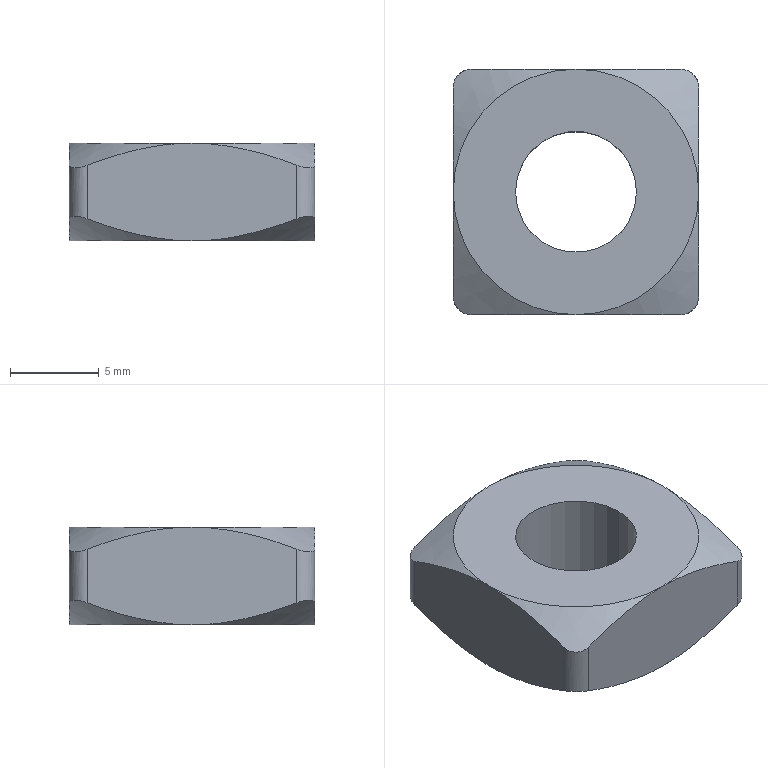Part | NX | features BREP 1 | 1 solid | 20 faces | box 13.8 x 13.8 x 5.5 mm | volume 804.819 mm3 | cone 8 | cylinder 6 | plane 6 | commonest cylinder face diameters 2 x4 6.8 x2
STEP:
#1=CARTESIAN_POINT('',(3.4,0.,-5.5));
#2=VERTEX_POINT('',#1);
#3=CARTESIAN_POINT('',(-3.4,0.,-5.5));
#4=VERTEX_POINT('',#3);
#5=CARTESIAN_POINT('',(0.,0.,-5.5));
#6=DIRECTION('',(0.,0.,1.));
#7=DIRECTION('',(1.,0.,0.));
#8=AXIS2_PLACEMENT_3D('',#5,#6,#7);
#9=CIRCLE('',#8,3.4);
#10=EDGE_CURVE('',#2,#4,#9,.T.);
#11=ORIENTED_EDGE('',*,*,#10,.F.);
#12=CARTESIAN_POINT('',(3.4,0.,0.));
#13=VERTEX_POINT('',#12);
#14=CARTESIAN_POINT('',(3.4,0.,0.));
#15=DIRECTION('',(0.,0.,1.));
#16=VECTOR('',#15,1000.);
#17=LINE('',#14,#16);
#18=EDGE_CURVE('',#2,#13,#17,.T.);
#19=ORIENTED_EDGE('',*,*,#18,.T.);
#20=CARTESIAN_POINT('',(-3.4,0.,0.));
#21=VERTEX_POINT('',#20);
#22=CARTESIAN_POINT('',(0.,0.,0.));
#23=DIRECTION('',(0.,0.,-1.));
#24=DIRECTION('',(-1.,0.,0.));
#25=AXIS2_PLACEMENT_3D('',#22,#23,#24);
#26=CIRCLE('',#25,3.4);
#27=EDGE_CURVE('',#21,#13,#26,.T.);
#28=ORIENTED_EDGE('',*,*,#27,.F.);
#29=CARTESIAN_POINT('',(-3.4,0.,0.));
#30=DIRECTION('',(0.,0.,1.));
#31=VECTOR('',#30,1000.);
#32=LINE('',#29,#31);
#33=EDGE_CURVE('',#4,#21,#32,.T.);
#34=ORIENTED_EDGE('',*,*,#33,.F.);
#35=EDGE_LOOP('',(#11,#19,#28,#34));
#36=FACE_BOUND('',#35,.T.);
#37=CARTESIAN_POINT('',(0.,0.,0.));
#38=DIRECTION('',(0.,0.,1.));
#39=DIRECTION('',(-1.,0.,0.));
#40=AXIS2_PLACEMENT_3D('',#37,#38,#39);
#41=CYLINDRICAL_SURFACE('',#40,3.4);
#42=ADVANCED_FACE('',(#36),#41,.F.);
#43=CARTESIAN_POINT('',(6.9,0.,0.));
#44=VERTEX_POINT('',#43);
#45=CARTESIAN_POINT('',(6.9,5.9,-1.245));
#46=VERTEX_POINT('',#45);
#47=CARTESIAN_POINT('',(6.9,5.9,-1.245));
#48=CARTESIAN_POINT('',(6.9,4.847,-0.854));
#49=CARTESIAN_POINT('',(6.9,3.07,-0.284));
#50=CARTESIAN_POINT('',(6.9,0.9944,0.));
#51=CARTESIAN_POINT('',(6.9,0.,0.));
#52=B_SPLINE_CURVE_WITH_KNOTS('',3,(#47,#48,#49,#50,#51),.UNSPECIFIED.,.F.,.F.,(4,1,4),(0.,0.5,1.),.UNSPECIFIED.);
#53=EDGE_CURVE('',#44,#46,#52,.F.);
#54=ORIENTED_EDGE('',*,*,#53,.F.);
#55=CARTESIAN_POINT('',(6.9,-5.9,-1.245));
#56=VERTEX_POINT('',#55);
#57=CARTESIAN_POINT('',(6.9,0.,0.));
#58=CARTESIAN_POINT('',(6.9,-0.4996,0.));
#59=CARTESIAN_POINT('',(6.9,-1.291,-0.05277));
#60=CARTESIAN_POINT('',(6.9,-2.234,-0.1946));
#61=CARTESIAN_POINT('',(6.9,-3.033,-0.3583));
#62=CARTESIAN_POINT('',(6.9,-3.663,-0.5175));
#63=CARTESIAN_POINT('',(6.9,-4.62,-0.792));
#64=CARTESIAN_POINT('',(6.9,-5.372,-1.049));
#65=CARTESIAN_POINT('',(6.9,-5.9,-1.245));
#66=B_SPLINE_CURVE_WITH_KNOTS('',3,(#57,#58,#59,#60,#61,#62,#63,#64,#65),.UNSPECIFIED.,.F.,.F.,(4,1,1,1,1,1,4),(0.,0.25,0.375,0.5,0.625,0.75,1.),.UNSPECIFIED.);
#67=EDGE_CURVE('',#56,#44,#66,.F.);
#68=ORIENTED_EDGE('',*,*,#67,.F.);
#69=CARTESIAN_POINT('',(6.9,-5.9,-4.255));
#70=VERTEX_POINT('',#69);
#71=CARTESIAN_POINT('',(6.9,-5.9,-5.5));
#72=DIRECTION('',(0.,0.,1.));
#73=VECTOR('',#72,1000.);
#74=LINE('',#71,#73);
#75=EDGE_CURVE('',#70,#56,#74,.T.);
#76=ORIENTED_EDGE('',*,*,#75,.F.);
#77=CARTESIAN_POINT('',(6.9,0.,-5.5));
#78=VERTEX_POINT('',#77);
#79=CARTESIAN_POINT('',(6.9,-5.9,-4.255));
#80=CARTESIAN_POINT('',(6.9,-4.851,-4.645));
#81=CARTESIAN_POINT('',(6.9,-3.084,-5.213));
#82=CARTESIAN_POINT('',(6.9,-0.9998,-5.5));
#83=CARTESIAN_POINT('',(6.9,0.,-5.5));
#84=B_SPLINE_CURVE_WITH_KNOTS('',3,(#79,#80,#81,#82,#83),.UNSPECIFIED.,.F.,.F.,(4,1,4),(0.,0.5,1.),.UNSPECIFIED.);
#85=EDGE_CURVE('',#78,#70,#84,.F.);
#86=ORIENTED_EDGE('',*,*,#85,.F.);
#87=CARTESIAN_POINT('',(6.9,5.9,-4.255));
#88=VERTEX_POINT('',#87);
#89=CARTESIAN_POINT('',(6.9,0.,-5.5));
#90=CARTESIAN_POINT('',(6.9,0.4969,-5.5));
#91=CARTESIAN_POINT('',(6.9,1.512,-5.437));
#92=CARTESIAN_POINT('',(6.9,3.03,-5.157));
#93=CARTESIAN_POINT('',(6.9,4.34,-4.8));
#94=CARTESIAN_POINT('',(6.9,5.37,-4.452));
#95=CARTESIAN_POINT('',(6.9,5.9,-4.255));
#96=B_SPLINE_CURVE_WITH_KNOTS('',3,(#89,#90,#91,#92,#93,#94,#95),.UNSPECIFIED.,.F.,.F.,(4,1,1,1,4),(0.,0.25,0.5,0.75,1.),.UNSPECIFIED.);
#97=EDGE_CURVE('',#88,#78,#96,.F.);
#98=ORIENTED_EDGE('',*,*,#97,.F.);
#99=CARTESIAN_POINT('',(6.9,5.9,-5.5));
#100=DIRECTION('',(0.,0.,-1.));
#101=VECTOR('',#100,1000.);
#102=LINE('',#99,#101);
#103=EDGE_CURVE('',#46,#88,#102,.T.);
#104=ORIENTED_EDGE('',*,*,#103,.F.);
#105=EDGE_LOOP('',(#54,#68,#76,#86,#98,#104));
#106=FACE_BOUND('',#105,.T.);
#107=CARTESIAN_POINT('',(6.9,6.9,-5.5));
#108=DIRECTION('',(-1.,0.,0.));
#109=DIRECTION('',(0.,1.,0.));
#110=AXIS2_PLACEMENT_3D('',#107,#108,#109);
#111=PLANE('',#110);
#112=ADVANCED_FACE('',(#106),#111,.F.);
#113=CARTESIAN_POINT('',(0.,6.9,-5.5));
#114=VERTEX_POINT('',#113);
#115=CARTESIAN_POINT('',(5.9,6.9,-4.255));
#116=VERTEX_POINT('',#115);
#117=CARTESIAN_POINT('',(5.9,6.9,-4.255));
#118=CARTESIAN_POINT('',(4.847,6.9,-4.646));
#119=CARTESIAN_POINT('',(3.07,6.9,-5.216));
#120=CARTESIAN_POINT('',(0.9944,6.9,-5.5));
#121=CARTESIAN_POINT('',(0.,6.9,-5.5));
#122=B_SPLINE_CURVE_WITH_KNOTS('',3,(#117,#118,#119,#120,#121),.UNSPECIFIED.,.F.,.F.,(4,1,4),(0.,0.5,1.),.UNSPECIFIED.);
#123=EDGE_CURVE('',#114,#116,#122,.F.);
#124=ORIENTED_EDGE('',*,*,#123,.F.);
#125=CARTESIAN_POINT('',(-5.9,6.9,-4.255));
#126=VERTEX_POINT('',#125);
#127=CARTESIAN_POINT('',(0.,6.9,-5.5));
#128=CARTESIAN_POINT('',(-0.4996,6.9,-5.5));
#129=CARTESIAN_POINT('',(-1.291,6.9,-5.447));
#130=CARTESIAN_POINT('',(-2.234,6.9,-5.305));
#131=CARTESIAN_POINT('',(-3.033,6.9,-5.142));
#132=CARTESIAN_POINT('',(-3.663,6.9,-4.983));
#133=CARTESIAN_POINT('',(-4.62,6.9,-4.708));
#134=CARTESIAN_POINT('',(-5.372,6.9,-4.451));
#135=CARTESIAN_POINT('',(-5.9,6.9,-4.255));
#136=B_SPLINE_CURVE_WITH_KNOTS('',3,(#127,#128,#129,#130,#131,#132,#133,#134,#135),.UNSPECIFIED.,.F.,.F.,(4,1,1,1,1,1,4),(0.,0.25,0.375,0.5,0.625,0.75,1.),.UNSPECIFIED.);
#137=EDGE_CURVE('',#126,#114,#136,.F.);
#138=ORIENTED_EDGE('',*,*,#137,.F.);
#139=CARTESIAN_POINT('',(-5.9,6.9,-1.245));
#140=VERTEX_POINT('',#139);
#141=CARTESIAN_POINT('',(-5.9,6.9,-5.5));
#142=DIRECTION('',(0.,0.,-1.));
#143=VECTOR('',#142,1000.);
#144=LINE('',#141,#143);
#145=EDGE_CURVE('',#140,#126,#144,.T.);
#146=ORIENTED_EDGE('',*,*,#145,.F.);
#147=CARTESIAN_POINT('',(0.,6.9,0.));
#148=VERTEX_POINT('',#147);
#149=CARTESIAN_POINT('',(-5.9,6.9,-1.245));
#150=CARTESIAN_POINT('',(-4.851,6.9,-0.8553));
#151=CARTESIAN_POINT('',(-3.084,6.9,-0.2875));
#152=CARTESIAN_POINT('',(-0.9998,6.9,0.));
#153=CARTESIAN_POINT('',(0.,6.9,0.));
#154=B_SPLINE_CURVE_WITH_KNOTS('',3,(#149,#150,#151,#152,#153),.UNSPECIFIED.,.F.,.F.,(4,1,4),(0.,0.5,1.),.UNSPECIFIED.);
#155=EDGE_CURVE('',#148,#140,#154,.F.);
#156=ORIENTED_EDGE('',*,*,#155,.F.);
#157=CARTESIAN_POINT('',(5.9,6.9,-1.245));
#158=VERTEX_POINT('',#157);
#159=CARTESIAN_POINT('',(0.,6.9,0.));
#160=CARTESIAN_POINT('',(0.4969,6.9,0.));
#161=CARTESIAN_POINT('',(1.512,6.9,-0.06256));
#162=CARTESIAN_POINT('',(3.03,6.9,-0.3426));
#163=CARTESIAN_POINT('',(4.34,6.9,-0.7001));
#164=CARTESIAN_POINT('',(5.37,6.9,-1.048));
#165=CARTESIAN_POINT('',(5.9,6.9,-1.245));
#166=B_SPLINE_CURVE_WITH_KNOTS('',3,(#159,#160,#161,#162,#163,#164,#165),.UNSPECIFIED.,.F.,.F.,(4,1,1,1,4),(0.,0.25,0.5,0.75,1.),.UNSPECIFIED.);
#167=EDGE_CURVE('',#158,#148,#166,.F.);
#168=ORIENTED_EDGE('',*,*,#167,.F.);
#169=CARTESIAN_POINT('',(5.9,6.9,-5.5));
#170=DIRECTION('',(0.,0.,1.));
#171=VECTOR('',#170,1000.);
#172=LINE('',#169,#171);
#173=EDGE_CURVE('',#116,#158,#172,.T.);
#174=ORIENTED_EDGE('',*,*,#173,.F.);
#175=EDGE_LOOP('',(#124,#138,#146,#156,#168,#174));
#176=FACE_BOUND('',#175,.T.);
#177=CARTESIAN_POINT('',(-6.9,6.9,-5.5));
#178=DIRECTION('',(0.,-1.,0.));
#179=DIRECTION('',(0.,0.,-1.));
#180=AXIS2_PLACEMENT_3D('',#177,#178,#179);
#181=PLANE('',#180);
#182=ADVANCED_FACE('',(#176),#181,.F.);
#183=CARTESIAN_POINT('',(-6.9,0.,0.));
#184=VERTEX_POINT('',#183);
#185=CARTESIAN_POINT('',(-6.9,-5.9,-1.245));
#186=VERTEX_POINT('',#185);
#187=CARTESIAN_POINT('',(-6.9,-5.9,-1.245));
#188=CARTESIAN_POINT('',(-6.9,-4.851,-0.8553));
#189=CARTESIAN_POINT('',(-6.9,-3.084,-0.2875));
#190=CARTESIAN_POINT('',(-6.9,-0.9998,0.));
#191=CARTESIAN_POINT('',(-6.9,0.,0.));
#192=B_SPLINE_CURVE_WITH_KNOTS('',3,(#187,#188,#189,#190,#191),.UNSPECIFIED.,.F.,.F.,(4,1,4),(0.,0.5,1.),.UNSPECIFIED.);
#193=EDGE_CURVE('',#184,#186,#192,.F.);
#194=ORIENTED_EDGE('',*,*,#193,.F.);
#195=CARTESIAN_POINT('',(-6.9,5.9,-1.245));
#196=VERTEX_POINT('',#195);
#197=CARTESIAN_POINT('',(-6.9,0.,0.));
#198=CARTESIAN_POINT('',(-6.9,0.4969,0.));
#199=CARTESIAN_POINT('',(-6.9,1.512,-0.06256));
#200=CARTESIAN_POINT('',(-6.9,3.03,-0.3426));
#201=CARTESIAN_POINT('',(-6.9,4.34,-0.7001));
#202=CARTESIAN_POINT('',(-6.9,5.37,-1.048));
#203=CARTESIAN_POINT('',(-6.9,5.9,-1.245));
#204=B_SPLINE_CURVE_WITH_KNOTS('',3,(#197,#198,#199,#200,#201,#202,#203),.UNSPECIFIED.,.F.,.F.,(4,1,1,1,4),(0.,0.25,0.5,0.75,1.),.UNSPECIFIED.);
#205=EDGE_CURVE('',#196,#184,#204,.F.);
#206=ORIENTED_EDGE('',*,*,#205,.F.);
#207=CARTESIAN_POINT('',(-6.9,5.9,-4.255));
#208=VERTEX_POINT('',#207);
#209=CARTESIAN_POINT('',(-6.9,5.9,-5.5));
#210=DIRECTION('',(0.,0.,1.));
#211=VECTOR('',#210,1000.);
#212=LINE('',#209,#211);
#213=EDGE_CURVE('',#208,#196,#212,.T.);
#214=ORIENTED_EDGE('',*,*,#213,.F.);
#215=CARTESIAN_POINT('',(-6.9,0.,-5.5));
#216=VERTEX_POINT('',#215);
#217=CARTESIAN_POINT('',(-6.9,5.9,-4.255));
#218=CARTESIAN_POINT('',(-6.9,4.847,-4.646));
#219=CARTESIAN_POINT('',(-6.9,3.07,-5.216));
#220=CARTESIAN_POINT('',(-6.9,0.9944,-5.5));
#221=CARTESIAN_POINT('',(-6.9,0.,-5.5));
#222=B_SPLINE_CURVE_WITH_KNOTS('',3,(#217,#218,#219,#220,#221),.UNSPECIFIED.,.F.,.F.,(4,1,4),(0.,0.5,1.),.UNSPECIFIED.);
#223=EDGE_CURVE('',#216,#208,#222,.F.);
#224=ORIENTED_EDGE('',*,*,#223,.F.);
#225=CARTESIAN_POINT('',(-6.9,-5.9,-4.255));
#226=VERTEX_POINT('',#225);
#227=CARTESIAN_POINT('',(-6.9,0.,-5.5));
#228=CARTESIAN_POINT('',(-6.9,-0.4996,-5.5));
#229=CARTESIAN_POINT('',(-6.9,-1.291,-5.447));
#230=CARTESIAN_POINT('',(-6.9,-2.234,-5.305));
#231=CARTESIAN_POINT('',(-6.9,-3.033,-5.142));
#232=CARTESIAN_POINT('',(-6.9,-3.663,-4.983));
#233=CARTESIAN_POINT('',(-6.9,-4.62,-4.708));
#234=CARTESIAN_POINT('',(-6.9,-5.372,-4.451));
#235=CARTESIAN_POINT('',(-6.9,-5.9,-4.255));
#236=B_SPLINE_CURVE_WITH_KNOTS('',3,(#227,#228,#229,#230,#231,#232,#233,#234,#235),.UNSPECIFIED.,.F.,.F.,(4,1,1,1,1,1,4),(0.,0.25,0.375,0.5,0.625,0.75,1.),.UNSPECIFIED.);
#237=EDGE_CURVE('',#226,#216,#236,.F.);
#238=ORIENTED_EDGE('',*,*,#237,.F.);
#239=CARTESIAN_POINT('',(-6.9,-5.9,-5.5));
#240=DIRECTION('',(0.,0.,-1.));
#241=VECTOR('',#240,1000.);
#242=LINE('',#239,#241);
#243=EDGE_CURVE('',#186,#226,#242,.T.);
#244=ORIENTED_EDGE('',*,*,#243,.F.);
#245=EDGE_LOOP('',(#194,#206,#214,#224,#238,#244));
#246=FACE_BOUND('',#245,.T.);
#247=CARTESIAN_POINT('',(-6.9,6.9,-5.5));
#248=DIRECTION('',(1.,0.,0.));
#249=DIRECTION('',(0.,1.,0.));
#250=AXIS2_PLACEMENT_3D('',#247,#248,#249);
#251=PLANE('',#250);
#252=ADVANCED_FACE('',(#246),#251,.F.);
#253=CARTESIAN_POINT('',(0.,-6.9,-5.5));
#254=VERTEX_POINT('',#253);
#255=CARTESIAN_POINT('',(-5.9,-6.9,-4.255));
#256=VERTEX_POINT('',#255);
#257=CARTESIAN_POINT('',(-5.9,-6.9,-4.255));
#258=CARTESIAN_POINT('',(-4.851,-6.9,-4.645));
#259=CARTESIAN_POINT('',(-3.084,-6.9,-5.213));
#260=CARTESIAN_POINT('',(-0.9998,-6.9,-5.5));
#261=CARTESIAN_POINT('',(0.,-6.9,-5.5));
#262=B_SPLINE_CURVE_WITH_KNOTS('',3,(#257,#258,#259,#260,#261),.UNSPECIFIED.,.F.,.F.,(4,1,4),(0.,0.5,1.),.UNSPECIFIED.);
#263=EDGE_CURVE('',#254,#256,#262,.F.);
#264=ORIENTED_EDGE('',*,*,#263,.F.);
#265=CARTESIAN_POINT('',(5.9,-6.9,-4.255));
#266=VERTEX_POINT('',#265);
#267=CARTESIAN_POINT('',(0.,-6.9,-5.5));
#268=CARTESIAN_POINT('',(0.4969,-6.9,-5.5));
#269=CARTESIAN_POINT('',(1.512,-6.9,-5.437));
#270=CARTESIAN_POINT('',(3.03,-6.9,-5.157));
#271=CARTESIAN_POINT('',(4.34,-6.9,-4.8));
#272=CARTESIAN_POINT('',(5.37,-6.9,-4.452));
#273=CARTESIAN_POINT('',(5.9,-6.9,-4.255));
#274=B_SPLINE_CURVE_WITH_KNOTS('',3,(#267,#268,#269,#270,#271,#272,#273),.UNSPECIFIED.,.F.,.F.,(4,1,1,1,4),(0.,0.25,0.5,0.75,1.),.UNSPECIFIED.);
#275=EDGE_CURVE('',#266,#254,#274,.F.);
#276=ORIENTED_EDGE('',*,*,#275,.F.);
#277=CARTESIAN_POINT('',(5.9,-6.9,-1.245));
#278=VERTEX_POINT('',#277);
#279=CARTESIAN_POINT('',(5.9,-6.9,-5.5));
#280=DIRECTION('',(0.,0.,-1.));
#281=VECTOR('',#280,1000.);
#282=LINE('',#279,#281);
#283=EDGE_CURVE('',#278,#266,#282,.T.);
#284=ORIENTED_EDGE('',*,*,#283,.F.);
#285=CARTESIAN_POINT('',(0.,-6.9,0.));
#286=VERTEX_POINT('',#285);
#287=CARTESIAN_POINT('',(5.9,-6.9,-1.245));
#288=CARTESIAN_POINT('',(4.847,-6.9,-0.854));
#289=CARTESIAN_POINT('',(3.07,-6.9,-0.284));
#290=CARTESIAN_POINT('',(0.9944,-6.9,0.));
#291=CARTESIAN_POINT('',(0.,-6.9,0.));
#292=B_SPLINE_CURVE_WITH_KNOTS('',3,(#287,#288,#289,#290,#291),.UNSPECIFIED.,.F.,.F.,(4,1,4),(0.,0.5,1.),.UNSPECIFIED.);
#293=EDGE_CURVE('',#286,#278,#292,.F.);
#294=ORIENTED_EDGE('',*,*,#293,.F.);
#295=CARTESIAN_POINT('',(-5.9,-6.9,-1.245));
#296=VERTEX_POINT('',#295);
#297=CARTESIAN_POINT('',(0.,-6.9,0.));
#298=CARTESIAN_POINT('',(-0.4996,-6.9,0.));
#299=CARTESIAN_POINT('',(-1.291,-6.9,-0.05277));
#300=CARTESIAN_POINT('',(-2.234,-6.9,-0.1946));
#301=CARTESIAN_POINT('',(-3.033,-6.9,-0.3583));
#302=CARTESIAN_POINT('',(-3.663,-6.9,-0.5175));
#303=CARTESIAN_POINT('',(-4.62,-6.9,-0.792));
#304=CARTESIAN_POINT('',(-5.372,-6.9,-1.049));
#305=CARTESIAN_POINT('',(-5.9,-6.9,-1.245));
#306=B_SPLINE_CURVE_WITH_KNOTS('',3,(#297,#298,#299,#300,#301,#302,#303,#304,#305),.UNSPECIFIED.,.F.,.F.,(4,1,1,1,1,1,4),(0.,0.25,0.375,0.5,0.625,0.75,1.),.UNSPECIFIED.);
#307=EDGE_CURVE('',#296,#286,#306,.F.);
#308=ORIENTED_EDGE('',*,*,#307,.F.);
#309=CARTESIAN_POINT('',(-5.9,-6.9,-5.5));
#310=DIRECTION('',(0.,0.,1.));
#311=VECTOR('',#310,1000.);
#312=LINE('',#309,#311);
#313=EDGE_CURVE('',#256,#296,#312,.T.);
#314=ORIENTED_EDGE('',*,*,#313,.F.);
#315=EDGE_LOOP('',(#264,#276,#284,#294,#308,#314));
#316=FACE_BOUND('',#315,.T.);
#317=CARTESIAN_POINT('',(-6.9,-6.9,-5.5));
#318=DIRECTION('',(0.,1.,0.));
#319=DIRECTION('',(1.,0.,0.));
#320=AXIS2_PLACEMENT_3D('',#317,#318,#319);
#321=PLANE('',#320);
#322=ADVANCED_FACE('',(#316),#321,.F.);
#323=CARTESIAN_POINT('',(0.,0.,-5.5));
#324=DIRECTION('',(0.,0.,-1.));
#325=DIRECTION('',(1.,0.,0.));
#326=AXIS2_PLACEMENT_3D('',#323,#324,#325);
#327=CIRCLE('',#326,6.9);
#328=EDGE_CURVE('',#78,#254,#327,.T.);
#329=ORIENTED_EDGE('',*,*,#328,.T.);
#330=CARTESIAN_POINT('',(0.,0.,-5.5));
#331=DIRECTION('',(0.,0.,-1.));
#332=DIRECTION('',(1.,0.,0.));
#333=AXIS2_PLACEMENT_3D('',#330,#331,#332);
#334=CIRCLE('',#333,6.9);
#335=EDGE_CURVE('',#254,#216,#334,.T.);
#336=ORIENTED_EDGE('',*,*,#335,.T.);
#337=CARTESIAN_POINT('',(0.,0.,-5.5));
#338=DIRECTION('',(0.,0.,-1.));
#339=DIRECTION('',(-1.,0.,0.));
#340=AXIS2_PLACEMENT_3D('',#337,#338,#339);
#341=CIRCLE('',#340,6.9);
#342=EDGE_CURVE('',#216,#114,#341,.T.);
#343=ORIENTED_EDGE('',*,*,#342,.T.);
#344=CARTESIAN_POINT('',(0.,0.,-5.5));
#345=DIRECTION('',(0.,0.,-1.));
#346=DIRECTION('',(1.,0.,0.));
#347=AXIS2_PLACEMENT_3D('',#344,#345,#346);
#348=CIRCLE('',#347,6.9);
#349=EDGE_CURVE('',#114,#78,#348,.T.);
#350=ORIENTED_EDGE('',*,*,#349,.T.);
#351=EDGE_LOOP('',(#329,#336,#343,#350));
#352=FACE_BOUND('',#351,.T.);
#353=CARTESIAN_POINT('',(0.,0.,-5.5));
#354=DIRECTION('',(0.,0.,1.));
#355=DIRECTION('',(1.,0.,0.));
#356=AXIS2_PLACEMENT_3D('',#353,#354,#355);
#357=CIRCLE('',#356,3.4);
#358=EDGE_CURVE('',#4,#2,#357,.T.);
#359=ORIENTED_EDGE('',*,*,#358,.T.);
#360=ORIENTED_EDGE('',*,*,#10,.T.);
#361=EDGE_LOOP('',(#359,#360));
#362=FACE_BOUND('',#361,.T.);
#363=CARTESIAN_POINT('',(0.,0.,-5.5));
#364=DIRECTION('',(0.,0.,-1.));
#365=DIRECTION('',(0.,-1.,0.));
#366=AXIS2_PLACEMENT_3D('',#363,#364,#365);
#367=PLANE('',#366);
#368=ADVANCED_FACE('',(#352,#362),#367,.T.);
#369=CARTESIAN_POINT('',(0.,0.,0.));
#370=DIRECTION('',(0.,0.,-1.));
#371=DIRECTION('',(1.,0.,0.));
#372=AXIS2_PLACEMENT_3D('',#369,#370,#371);
#373=CIRCLE('',#372,6.9);
#374=EDGE_CURVE('',#148,#44,#373,.T.);
#375=ORIENTED_EDGE('',*,*,#374,.F.);
#376=CARTESIAN_POINT('',(0.,0.,0.));
#377=DIRECTION('',(0.,0.,-1.));
#378=DIRECTION('',(-1.,0.,0.));
#379=AXIS2_PLACEMENT_3D('',#376,#377,#378);
#380=CIRCLE('',#379,6.9);
#381=EDGE_CURVE('',#184,#148,#380,.T.);
#382=ORIENTED_EDGE('',*,*,#381,.F.);
#383=CARTESIAN_POINT('',(0.,0.,0.));
#384=DIRECTION('',(0.,0.,-1.));
#385=DIRECTION('',(1.,0.,0.));
#386=AXIS2_PLACEMENT_3D('',#383,#384,#385);
#387=CIRCLE('',#386,6.9);
#388=EDGE_CURVE('',#286,#184,#387,.T.);
#389=ORIENTED_EDGE('',*,*,#388,.F.);
#390=CARTESIAN_POINT('',(0.,0.,0.));
#391=DIRECTION('',(0.,0.,-1.));
#392=DIRECTION('',(1.,0.,0.));
#393=AXIS2_PLACEMENT_3D('',#390,#391,#392);
#394=CIRCLE('',#393,6.9);
#395=EDGE_CURVE('',#44,#286,#394,.T.);
#396=ORIENTED_EDGE('',*,*,#395,.F.);
#397=EDGE_LOOP('',(#375,#382,#389,#396));
#398=FACE_BOUND('',#397,.T.);
#399=ORIENTED_EDGE('',*,*,#27,.T.);
#400=CARTESIAN_POINT('',(0.,0.,0.));
#401=DIRECTION('',(0.,0.,-1.));
#402=DIRECTION('',(-1.,0.,0.));
#403=AXIS2_PLACEMENT_3D('',#400,#401,#402);
#404=CIRCLE('',#403,3.4);
#405=EDGE_CURVE('',#13,#21,#404,.T.);
#406=ORIENTED_EDGE('',*,*,#405,.T.);
#407=EDGE_LOOP('',(#399,#406));
#408=FACE_BOUND('',#407,.T.);
#409=CARTESIAN_POINT('',(0.,0.,0.));
#410=DIRECTION('',(0.,0.,-1.));
#411=DIRECTION('',(0.,-1.,0.));
#412=AXIS2_PLACEMENT_3D('',#409,#410,#411);
#413=PLANE('',#412);
#414=ADVANCED_FACE('',(#398,#408),#413,.F.);
#415=ORIENTED_EDGE('',*,*,#18,.F.);
#416=ORIENTED_EDGE('',*,*,#358,.F.);
#417=ORIENTED_EDGE('',*,*,#33,.T.);
#418=ORIENTED_EDGE('',*,*,#405,.F.);
#419=EDGE_LOOP('',(#415,#416,#417,#418));
#420=FACE_BOUND('',#419,.T.);
#421=CARTESIAN_POINT('',(0.,0.,0.));
#422=DIRECTION('',(0.,0.,1.));
#423=DIRECTION('',(-1.,0.,0.));
#424=AXIS2_PLACEMENT_3D('',#421,#422,#423);
#425=CYLINDRICAL_SURFACE('',#424,3.4);
#426=ADVANCED_FACE('',(#420),#425,.F.);
#427=ORIENTED_EDGE('',*,*,#167,.T.);
#428=ORIENTED_EDGE('',*,*,#374,.T.);
#429=ORIENTED_EDGE('',*,*,#53,.T.);
#430=CARTESIAN_POINT('',(5.9,6.9,-1.245));
#431=CARTESIAN_POINT('',(6.431,6.9,-1.442));
#432=CARTESIAN_POINT('',(6.9,6.431,-1.442));
#433=CARTESIAN_POINT('',(6.9,5.9,-1.245));
#434=B_SPLINE_CURVE_WITH_KNOTS('',3,(#430,#431,#432,#433),.UNSPECIFIED.,.F.,.F.,(4,4),(0.,1.),.UNSPECIFIED.);
#435=EDGE_CURVE('',#158,#46,#434,.T.);
#436=ORIENTED_EDGE('',*,*,#435,.F.);
#437=EDGE_LOOP('',(#427,#428,#429,#436));
#438=FACE_BOUND('',#437,.T.);
#439=CARTESIAN_POINT('',(0.,0.,-2.));
#440=DIRECTION('',(0.,0.,-1.));
#441=DIRECTION('',(1.,0.,0.));
#442=AXIS2_PLACEMENT_3D('',#439,#440,#441);
#443=CONICAL_SURFACE('',#442,10.4,1.052);
#444=ADVANCED_FACE('',(#438),#443,.T.);
#445=ORIENTED_EDGE('',*,*,#205,.T.);
#446=ORIENTED_EDGE('',*,*,#381,.T.);
#447=ORIENTED_EDGE('',*,*,#155,.T.);
#448=CARTESIAN_POINT('',(-6.9,5.9,-1.245));
#449=CARTESIAN_POINT('',(-6.9,6.431,-1.442));
#450=CARTESIAN_POINT('',(-6.431,6.9,-1.442));
#451=CARTESIAN_POINT('',(-5.9,6.9,-1.245));
#452=B_SPLINE_CURVE_WITH_KNOTS('',3,(#448,#449,#450,#451),.UNSPECIFIED.,.F.,.F.,(4,4),(0.,1.),.UNSPECIFIED.);
#453=EDGE_CURVE('',#196,#140,#452,.T.);
#454=ORIENTED_EDGE('',*,*,#453,.F.);
#455=EDGE_LOOP('',(#445,#446,#447,#454));
#456=FACE_BOUND('',#455,.T.);
#457=CARTESIAN_POINT('',(0.,0.,-2.));
#458=DIRECTION('',(0.,0.,-1.));
#459=DIRECTION('',(1.,0.,0.));
#460=AXIS2_PLACEMENT_3D('',#457,#458,#459);
#461=CONICAL_SURFACE('',#460,10.4,1.052);
#462=ADVANCED_FACE('',(#456),#461,.T.);
#463=ORIENTED_EDGE('',*,*,#307,.T.);
#464=ORIENTED_EDGE('',*,*,#388,.T.);
#465=ORIENTED_EDGE('',*,*,#193,.T.);
#466=CARTESIAN_POINT('',(-5.9,-6.9,-1.245));
#467=CARTESIAN_POINT('',(-6.431,-6.9,-1.442));
#468=CARTESIAN_POINT('',(-6.9,-6.431,-1.442));
#469=CARTESIAN_POINT('',(-6.9,-5.9,-1.245));
#470=B_SPLINE_CURVE_WITH_KNOTS('',3,(#466,#467,#468,#469),.UNSPECIFIED.,.F.,.F.,(4,4),(0.,1.),.UNSPECIFIED.);
#471=EDGE_CURVE('',#296,#186,#470,.T.);
#472=ORIENTED_EDGE('',*,*,#471,.F.);
#473=EDGE_LOOP('',(#463,#464,#465,#472));
#474=FACE_BOUND('',#473,.T.);
#475=CARTESIAN_POINT('',(0.,0.,-2.));
#476=DIRECTION('',(0.,0.,-1.));
#477=DIRECTION('',(1.,0.,0.));
#478=AXIS2_PLACEMENT_3D('',#475,#476,#477);
#479=CONICAL_SURFACE('',#478,10.4,1.052);
#480=ADVANCED_FACE('',(#474),#479,.T.);
#481=ORIENTED_EDGE('',*,*,#67,.T.);
#482=ORIENTED_EDGE('',*,*,#395,.T.);
#483=ORIENTED_EDGE('',*,*,#293,.T.);
#484=CARTESIAN_POINT('',(6.9,-5.9,-1.245));
#485=CARTESIAN_POINT('',(6.9,-6.431,-1.442));
#486=CARTESIAN_POINT('',(6.431,-6.9,-1.442));
#487=CARTESIAN_POINT('',(5.9,-6.9,-1.245));
#488=B_SPLINE_CURVE_WITH_KNOTS('',3,(#484,#485,#486,#487),.UNSPECIFIED.,.F.,.F.,(4,4),(0.,1.),.UNSPECIFIED.);
#489=EDGE_CURVE('',#56,#278,#488,.T.);
#490=ORIENTED_EDGE('',*,*,#489,.F.);
#491=EDGE_LOOP('',(#481,#482,#483,#490));
#492=FACE_BOUND('',#491,.T.);
#493=CARTESIAN_POINT('',(0.,0.,-2.));
#494=DIRECTION('',(0.,0.,-1.));
#495=DIRECTION('',(1.,0.,0.));
#496=AXIS2_PLACEMENT_3D('',#493,#494,#495);
#497=CONICAL_SURFACE('',#496,10.4,1.052);
#498=ADVANCED_FACE('',(#492),#497,.T.);
#499=ORIENTED_EDGE('',*,*,#97,.T.);
#500=ORIENTED_EDGE('',*,*,#349,.F.);
#501=ORIENTED_EDGE('',*,*,#123,.T.);
#502=CARTESIAN_POINT('',(6.9,5.9,-4.255));
#503=CARTESIAN_POINT('',(6.9,6.431,-4.058));
#504=CARTESIAN_POINT('',(6.431,6.9,-4.058));
#505=CARTESIAN_POINT('',(5.9,6.9,-4.255));
#506=B_SPLINE_CURVE_WITH_KNOTS('',3,(#502,#503,#504,#505),.UNSPECIFIED.,.F.,.F.,(4,4),(0.,1.),.UNSPECIFIED.);
#507=EDGE_CURVE('',#88,#116,#506,.T.);
#508=ORIENTED_EDGE('',*,*,#507,.F.);
#509=EDGE_LOOP('',(#499,#500,#501,#508));
#510=FACE_BOUND('',#509,.T.);
#511=CARTESIAN_POINT('',(0.,0.,-5.5));
#512=DIRECTION('',(0.,0.,1.));
#513=DIRECTION('',(-1.,0.,0.));
#514=AXIS2_PLACEMENT_3D('',#511,#512,#513);
#515=CONICAL_SURFACE('',#514,6.9,1.052);
#516=ADVANCED_FACE('',(#510),#515,.T.);
#517=ORIENTED_EDGE('',*,*,#137,.T.);
#518=ORIENTED_EDGE('',*,*,#342,.F.);
#519=ORIENTED_EDGE('',*,*,#223,.T.);
#520=CARTESIAN_POINT('',(-5.9,6.9,-4.255));
#521=CARTESIAN_POINT('',(-6.431,6.9,-4.058));
#522=CARTESIAN_POINT('',(-6.9,6.431,-4.058));
#523=CARTESIAN_POINT('',(-6.9,5.9,-4.255));
#524=B_SPLINE_CURVE_WITH_KNOTS('',3,(#520,#521,#522,#523),.UNSPECIFIED.,.F.,.F.,(4,4),(0.,1.),.UNSPECIFIED.);
#525=EDGE_CURVE('',#126,#208,#524,.T.);
#526=ORIENTED_EDGE('',*,*,#525,.F.);
#527=EDGE_LOOP('',(#517,#518,#519,#526));
#528=FACE_BOUND('',#527,.T.);
#529=CARTESIAN_POINT('',(0.,0.,-5.5));
#530=DIRECTION('',(0.,0.,1.));
#531=DIRECTION('',(-1.,0.,0.));
#532=AXIS2_PLACEMENT_3D('',#529,#530,#531);
#533=CONICAL_SURFACE('',#532,6.9,1.052);
#534=ADVANCED_FACE('',(#528),#533,.T.);
#535=ORIENTED_EDGE('',*,*,#237,.T.);
#536=ORIENTED_EDGE('',*,*,#335,.F.);
#537=ORIENTED_EDGE('',*,*,#263,.T.);
#538=CARTESIAN_POINT('',(-6.9,-5.9,-4.255));
#539=CARTESIAN_POINT('',(-6.9,-6.431,-4.058));
#540=CARTESIAN_POINT('',(-6.431,-6.9,-4.058));
#541=CARTESIAN_POINT('',(-5.9,-6.9,-4.255));
#542=B_SPLINE_CURVE_WITH_KNOTS('',3,(#538,#539,#540,#541),.UNSPECIFIED.,.F.,.F.,(4,4),(0.,1.),.UNSPECIFIED.);
#543=EDGE_CURVE('',#226,#256,#542,.T.);
#544=ORIENTED_EDGE('',*,*,#543,.F.);
#545=EDGE_LOOP('',(#535,#536,#537,#544));
#546=FACE_BOUND('',#545,.T.);
#547=CARTESIAN_POINT('',(0.,0.,-5.5));
#548=DIRECTION('',(0.,0.,1.));
#549=DIRECTION('',(-1.,0.,0.));
#550=AXIS2_PLACEMENT_3D('',#547,#548,#549);
#551=CONICAL_SURFACE('',#550,6.9,1.052);
#552=ADVANCED_FACE('',(#546),#551,.T.);
#553=ORIENTED_EDGE('',*,*,#275,.T.);
#554=ORIENTED_EDGE('',*,*,#328,.F.);
#555=ORIENTED_EDGE('',*,*,#85,.T.);
#556=CARTESIAN_POINT('',(5.9,-6.9,-4.255));
#557=CARTESIAN_POINT('',(6.431,-6.9,-4.058));
#558=CARTESIAN_POINT('',(6.9,-6.431,-4.058));
#559=CARTESIAN_POINT('',(6.9,-5.9,-4.255));
#560=B_SPLINE_CURVE_WITH_KNOTS('',3,(#556,#557,#558,#559),.UNSPECIFIED.,.F.,.F.,(4,4),(0.,1.),.UNSPECIFIED.);
#561=EDGE_CURVE('',#266,#70,#560,.T.);
#562=ORIENTED_EDGE('',*,*,#561,.F.);
#563=EDGE_LOOP('',(#553,#554,#555,#562));
#564=FACE_BOUND('',#563,.T.);
#565=CARTESIAN_POINT('',(0.,0.,-5.5));
#566=DIRECTION('',(0.,0.,1.));
#567=DIRECTION('',(-1.,0.,0.));
#568=AXIS2_PLACEMENT_3D('',#565,#566,#567);
#569=CONICAL_SURFACE('',#568,6.9,1.052);
#570=ADVANCED_FACE('',(#564),#569,.T.);
#571=ORIENTED_EDGE('',*,*,#507,.T.);
#572=ORIENTED_EDGE('',*,*,#173,.T.);
#573=ORIENTED_EDGE('',*,*,#435,.T.);
#574=ORIENTED_EDGE('',*,*,#103,.T.);
#575=EDGE_LOOP('',(#571,#572,#573,#574));
#576=FACE_BOUND('',#575,.T.);
#577=CARTESIAN_POINT('',(5.9,5.9,-5.5));
#578=DIRECTION('',(0.,0.,1.));
#579=DIRECTION('',(-1.,0.,0.));
#580=AXIS2_PLACEMENT_3D('',#577,#578,#579);
#581=CYLINDRICAL_SURFACE('',#580,1.);
#582=ADVANCED_FACE('',(#576),#581,.T.);
#583=ORIENTED_EDGE('',*,*,#543,.T.);
#584=ORIENTED_EDGE('',*,*,#313,.T.);
#585=ORIENTED_EDGE('',*,*,#471,.T.);
#586=ORIENTED_EDGE('',*,*,#243,.T.);
#587=EDGE_LOOP('',(#583,#584,#585,#586));
#588=FACE_BOUND('',#587,.T.);
#589=CARTESIAN_POINT('',(-5.9,-5.9,-5.5));
#590=DIRECTION('',(0.,0.,1.));
#591=DIRECTION('',(-1.,0.,0.));
#592=AXIS2_PLACEMENT_3D('',#589,#590,#591);
#593=CYLINDRICAL_SURFACE('',#592,1.);
#594=ADVANCED_FACE('',(#588),#593,.T.);
#595=ORIENTED_EDGE('',*,*,#561,.T.);
#596=ORIENTED_EDGE('',*,*,#75,.T.);
#597=ORIENTED_EDGE('',*,*,#489,.T.);
#598=ORIENTED_EDGE('',*,*,#283,.T.);
#599=EDGE_LOOP('',(#595,#596,#597,#598));
#600=FACE_BOUND('',#599,.T.);
#601=CARTESIAN_POINT('',(5.9,-5.9,-5.5));
#602=DIRECTION('',(0.,0.,1.));
#603=DIRECTION('',(-1.,0.,0.));
#604=AXIS2_PLACEMENT_3D('',#601,#602,#603);
#605=CYLINDRICAL_SURFACE('',#604,1.);
#606=ADVANCED_FACE('',(#600),#605,.T.);
#607=ORIENTED_EDGE('',*,*,#525,.T.);
#608=ORIENTED_EDGE('',*,*,#213,.T.);
#609=ORIENTED_EDGE('',*,*,#453,.T.);
#610=ORIENTED_EDGE('',*,*,#145,.T.);
#611=EDGE_LOOP('',(#607,#608,#609,#610));
#612=FACE_BOUND('',#611,.T.);
#613=CARTESIAN_POINT('',(-5.9,5.9,-5.5));
#614=DIRECTION('',(0.,0.,1.));
#615=DIRECTION('',(-1.,0.,0.));
#616=AXIS2_PLACEMENT_3D('',#613,#614,#615);
#617=CYLINDRICAL_SURFACE('',#616,1.);
#618=ADVANCED_FACE('',(#612),#617,.T.);
#619=CLOSED_SHELL('',(#42,#112,#182,#252,#322,#368,#414,#426,#444,#462,#480,#498,#516,#534,#552,#570,#582,#594,#606,#618));
#620=MANIFOLD_SOLID_BREP('',#619);
#621=(LENGTH_UNIT()NAMED_UNIT(*)SI_UNIT(.MILLI.,.METRE.));
#622=UNCERTAINTY_MEASURE_WITH_UNIT(LENGTH_MEASURE(0.0508),#621,'','');
#623=(NAMED_UNIT(*)PLANE_ANGLE_UNIT()SI_UNIT($,.RADIAN.));
#624=(NAMED_UNIT(*)SI_UNIT($,.STERADIAN.)SOLID_ANGLE_UNIT());
#625=(GEOMETRIC_REPRESENTATION_CONTEXT(3)GLOBAL_UNCERTAINTY_ASSIGNED_CONTEXT((#622))GLOBAL_UNIT_ASSIGNED_CONTEXT((#621,#623,#624))REPRESENTATION_CONTEXT('',''));
#626=ADVANCED_BREP_SHAPE_REPRESENTATION('',(#620),#625);